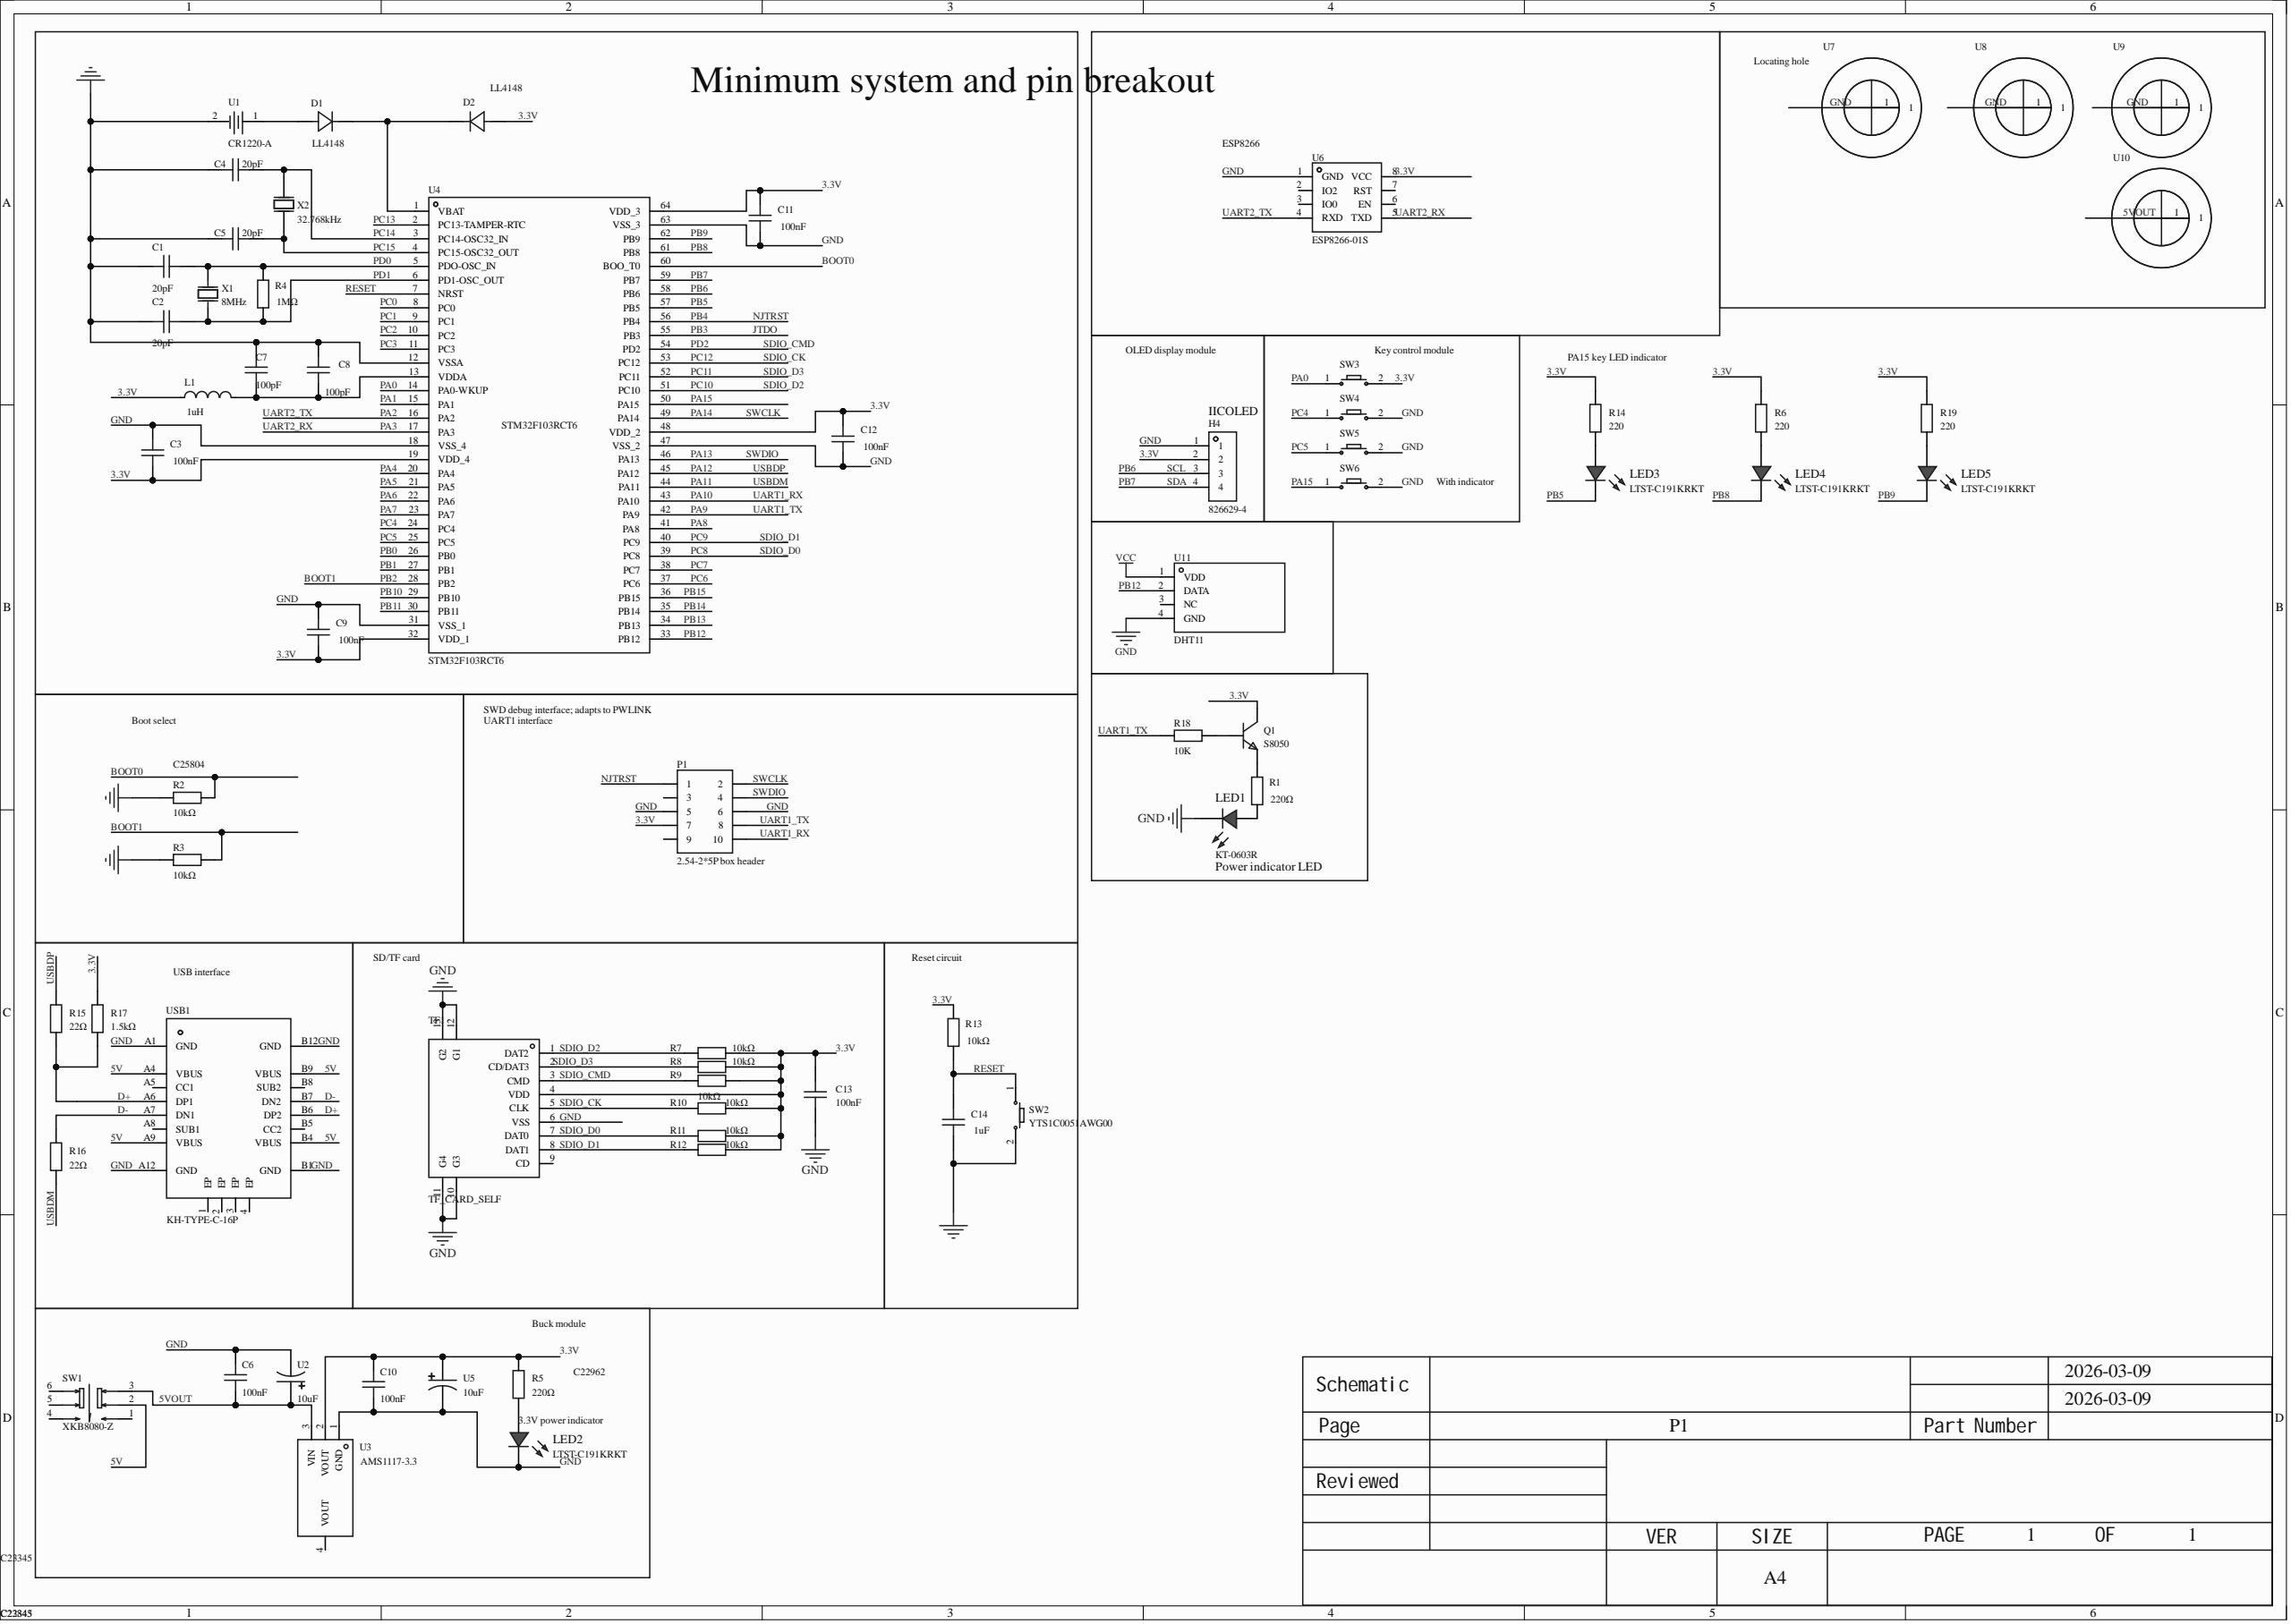Circuit board | Altium Designer | 65 parts | 48 nets
Bill of materials:
Comment,Description,Designator,Footprint,LibRef,Quantity
"20pF","Capacitance: 20pF; tolerance: ±5%; rated voltage: 50V; dielectric (temperature coefficient): C0G;","C1, C2, C4, C5","C0603","CL10C200JB8NNNC","4"
"100nF","Capacitance: 100nF; tolerance: ±10%; rated voltage: 50V; dielectric (temperature coefficient): X7R;","C3, C6, C9, C10, C11, C12, C13","C0603","CC0603KRX7R9BB104","7"
"100pF","Capacitance: 100pF; tolerance: ±5%; rated voltage: 50V; dielectric (temperature coefficient): C0G;","C7, C8","C0603","CL10C101JB8NNNC","2"
"1uF","Capacitance: 1uF; tolerance: ±10%; rated voltage: 50V; dielectric (temperature coefficient): X5R;","C14","C0603","CL10A105KB8NNNC","1"
"LL4148","","D1, D2","LL-34_L3.5-W1.5-RD","LL4148_C9808","2"
"826629-4","","H4","HDR-TH_4P-P2.54-V-M-1","826629-4","1"
"1uH","Inductance: 1uH; tolerance: ±20%; rated current: 1.7A; saturation current (Isat): 2.1A; DC resistance (DCR): 128mΩ;","L1","L0603","DFE18SAN1R0MG0L","1"
"KT-0603R","Emitted color: red; diode configuration: -; dominant wavelength: -; color temperature: -; power: -; mounting: -;","LED1","LED0603-RD","KT-0603R","1"
"LTST-C191KRKT","Emitted color: red; diode configuration: -; dominant wavelength: 631nm; color temperature: -; power: 75mW; mounting: -;","LED2, LED3, LED4, LED5","LED0603-RD","LTST-C191KRKT","4"
"2.54-2*5P box header","Connector type: box header; pins per row: 5; rows: 2; pitch: 2.54mm; row spacing: 2.54mm; package: through-hole; contact material: -; contact plating: -;","P1","IDC-TH_10P-P2.54_C5665","2.54-2*5P简牛","1"
"S8050","","Q1","SOT-23-3_L2.9-W1.3-P1.90-LS2.4-BR","S8050_C2762211","1"
"220Ω","","R1, R5","R0603","0603WAF2200T5E","2"
"10kΩ","","R2, R3, R7, R8, R9, R10, R11, R12, R13","R0603","0603WAF1002T5E","9"
"1MΩ","Resistor type: thick film resistor; resistance: 1MΩ; tolerance: ±1%; power: 100mW;","R4","R0603","0603WAF1004T5E","1"
"220","Resistor type: thick film resistor; resistance: 10kΩ; tolerance: ±1%; power: 100mW;","R6, R14, R19","R0603","0603WAF1002T5E","3"
"22Ω","Resistor type: thick film resistor; resistance: 22Ω; tolerance: ±1%; power: 100mW;","R15, R16","R0603","0603WAF220JT5E","2"
"1.5kΩ","Resistor type: thick film resistor; resistance: 1.5kΩ; tolerance: ±1%; power: 100mW;","R17","R0603","0603WAF1501T5E","1"
"10K","","R18","R0603","Res_0603","1"
"XKB8080-Z","","SW1","SW-TH_6P-L8.0-W8.0-P2.50","XKB8080-Z","1"
"YTS1C0051AWG00","Switch length: 6.1mm; switch width: 3.6mm; switch height: 2.5mm;","SW2, SW3, SW4, SW5, SW6","SW-SMD_L6.1-W3.6-LS8.0","YTS1C0051AWG00","5"
"TF_CARD_SELF","","TF1","TF-SMD_TF-15-15","TF_CARD_SELF","1"
"CR1220-A","","U1","BAT-SMD_CR1220-2","CR1220-A","1"
"10uF","","U2, U5","CASE-A_3216","NOJA106M006RWJ","2"
"AMS1117-3.3","Output type: fixed; output polarity: positive; output channels: 1; max input voltage: -; output voltage: 3.3V; dropout: 1.3V@(800mA); quiescent current (ground current): -; output current: 1A; power supply ripple rejection (PSRR): 72dB@(120Hz); noise: -; features: -; operating temperature: -;","U3","SOT-223-3_L6.5-W3.4-P2.30-LS7.0-BR","AMS1117-3.3_C6186","1"
"STM32F103RCT6","","U4","LQFP-64_L10.0-W10.0-P0.50-LS12.0-BL","STM32F103RCT6","1"
"ESP8266-01S","","U6","WIFIM-TH_ESP8266-01S","ESP8266-01S","1"
"","","U7, U8, U9, U10","M3_花孔","M3孔_花孔","4"
"DHT11","","U11","SENSOR-TH_DHT11","DHT11","1"
"KH-TYPE-C-16P","","USB1","USB-C-SMD_KH-TYPE-C-16P","KH-TYPE-C-16P","1"
"8MHz","","X1","HC-49S_L11.4-W4.8","X49SM8MSB2SC","1"
"32.768kHz","Frequency: 32.768kHz; frequency tolerance: ±20ppm; load capacitance: 12.5pF;","X2","OSC-TH_BD2.0-P0.70-D0.3","7S032768NW2","1"
Netlist (Protel format):
[
C1
C0603
20pF



]
[
C2
C0603
20pF



]
[
C3
C0603
100nF



]
[
C4
C0603
20pF



]
[
C5
C0603
20pF



]
[
C6
C0603
100nF



]
[
C7
C0603
100pF



]
[
C8
C0603
100pF



]
[
C9
C0603
100nF



]
[
C10
C0603
100nF



]
[
C11
C0603
100nF



]
[
C12
C0603
100nF



]
[
C13
C0603
100nF



]
[
C14
C0603
1uF



]
[
D1
LL-34_L3.5-W1.5-RD
LL4148



]
[
D2
LL-34_L3.5-W1.5-RD
LL4148



]
[
H4
HDR-TH_4P-P2.54-V-M-1
826629-4



]
[
L1
L0603
1uH



]
[
LED1
LED0603-RD
KT-0603R



]
[
LED2
LED0603-RD
LTST-C191KRKT



]
[
LED3
LED0603-RD
LTST-C191KRKT



]
[
LED4
LED0603-RD
LTST-C191KRKT



]
[
LED5
LED0603-RD
LTST-C191KRKT



]
[
P1
IDC-TH_10P-P2.54_C5665
2.54-2*5P box header



]
[
Q1
SOT-23-3_L2.9-W1.3-P1.90-LS2.4-BR
S8050



]
[
R1
R0603
220Ω



]
[
R2
R0603
10kΩ



]
[
R3
R0603
10kΩ



]
[
R4
R0603
1MΩ



]
[
R5
R0603
220Ω



]
[
R6
R0603
220



]
[
R7
R0603
10kΩ



]
[
R8
R0603
10kΩ



]
[
R9
R0603
10kΩ



]
[
R10
R0603
10kΩ



]
[
R11
R0603
10kΩ



]
[
R12
R0603
10kΩ



]
[
R13
R0603
10kΩ



]
[
R14
R0603
220



]
[
R15
R0603
22Ω



]
[
R16
R0603
22Ω



]
[
R17
R0603
1.5kΩ



]
[
R18
R0603
10K



]
[
R19
R0603
220



]
[
SW1
SW-TH_6P-L8.0-W8.0-P2.50
XKB8080-Z



]
[
SW2
SW-SMD_L6.1-W3.6-LS8.0
YTS1C0051AWG00



]
[
SW3
SW-SMD_L6.1-W3.6-LS8.0
YTS1C0051AWG00



]
[
SW4
SW-SMD_L6.1-W3.6-LS8.0
YTS1C0051AWG00



]
[
SW5
SW-SMD_L6.1-W3.6-LS8.0
YTS1C0051AWG00



]
[
SW6
SW-SMD_L6.1-W3.6-LS8.0
YTS1C0051AWG00



]
[
TF1
TF-SMD_TF-15-15
TF_CARD_SELF



]
[
U1
BAT-SMD_CR1220-2
CR1220-A



]
[
U2
CASE-A_3216
10uF



]
[
U3
SOT-223-3_L6.5-W3.4-P2.30-LS7.0-BR
AMS1117-3.3



]
[
U4
LQFP-64_L10.0-W10.0-P0.50-LS12.0-BL
STM32F103RCT6



]
[
U5
CASE-A_3216
10uF



]
[
U6
WIFIM-TH_ESP8266-01S
ESP8266-01S



]
[
U7
M3_花孔




]
[
U8
M3_花孔




]
[
U9
M3_花孔




]
[
U10
M3_花孔




]
[
U11
SENSOR-TH_DHT11
DHT11



]
[
USB1
USB-C-SMD_KH-TYPE-C-16P
KH-TYPE-C-16P



]
[
X1
HC-49S_L11.4-W4.8
8MHz



]
[
X2
OSC-TH_BD2.0-P0.70-D0.3
32.768kHz



]
(
RESET
C14-2
R13-1
SW2-1
U4-7
)
(
PD2
R9-1
TF1-3
U4-54
)
(
PD1
C2-2
R4-1
U4-6
X1-1
)
(
PD0
C1-2
R4-2
U4-5
X1-2
)
(
PC15
C5-2
U4-4
X2-2
)
(
PC14
C4-2
U4-3
X2-1
)
(
PC12
R10-1
TF1-5
U4-53
)
(
PC11
R8-1
TF1-2
U4-52
)
(
PC10
R7-1
TF1-1
U4-51
)
(
PC9
R12-1
TF1-8
U4-40
)
(
PC8
R11-1
TF1-7
U4-39
)
(
PC5
SW5-1
U4-25
)
(
PC4
SW4-1
U4-24
)
(
PB12
U4-33
U11-2
)
(
PB9
LED5-1
U4-62
)
(
PB8
LED4-1
U4-61
)
(
PB7
H4-4
U4-59
)
(
PB6
H4-3
U4-58
)
(
PB5
LED3-1
U4-57
)
(
PA15
SW6-1
U4-50
)
(
PA14
P1-2
U4-49
)
(
PA13
P1-4
U4-46
)
(
PA12
R15-2
U4-45
)
(
PA11
R16-1
U4-44
)
(
PA10
P1-10
U4-43
)
(
PA9
P1-8
R18-1
U4-42
)
(
PA3
U4-17
U6-5
)
(
PA2
U4-16
U6-4
)
(
PA0
SW3-1
U4-14
)
(
NJTRST
P1-1
U4-56
)
(
NetQ1_2
Q1-2
R1-2
)
(
NetQ1_1
Q1-1
R18-2
)
(
NetLED5_2
LED5-2
R19-1
)
(
NetLED4_2
LED4-2
R6-1
)
(
NetLED3_2
LED3-2
R14-1
)
(
NetLED2_2
LED2-2
R5-1
)
(
NetLED1_2
LED1-2
R1-1
)
(
NetD1_2
D1-2
U1-1
)
(
NetD1_1
D1-1
D2-1
U4-1
)
(
NetC7_1
C7-1
C8-1
L1-2
U4-13
)
(
GND
C1-1
C2-1
C3-2
C4-1
C5-1
C6-2
C7-2
C8-2
C9-2
C10-1
C11-1
C12-1
C13-1
C14-1
H4-1
LED1-1
LED2-1
P1-5
P1-6
R2-1
R3-1
SW2-2
SW4-2
SW5-2
SW6-2
TF1-6
TF1-10
TF1-11
TF1-12
TF1-13
U1-2
U2-2
U3-1
U4-12
U4-18
U4-31
U4-47
U4-63
U5-2
U6-1
U7-1
U8-1
U9-1
U11-4
USB1-A1
USB1-A12
USB1-B1
USB1-B12
)
(
D-
R16-2
USB1-A7
USB1-B7
)
(
D+
R15-1
R17-1
USB1-A6
USB1-B6
)
(
BOOT1
R3-2
U4-28
)
(
BOOT0
R2-2
U4-60
)
(
5VOUT
C6-1
SW1-3
U2-1
U3-3
U10-1
)
(
5V
SW1-2
USB1-A4
USB1-A9
USB1-B4
USB1-B9
)
(
3.3V
C3-1
C9-1
C10-2
C11-2
C12-2
C13-2
D2-2
H4-2
L1-1
P1-7
Q1-3
R5-2
R6-2
R7-2
R8-2
R9-2
R10-2
R11-2
R12-2
R13-2
R14-2
R17-2
R19-2
SW3-2
TF1-4
U3-2
U4-19
U4-32
U4-48
U4-64
U5-1
U6-8
)